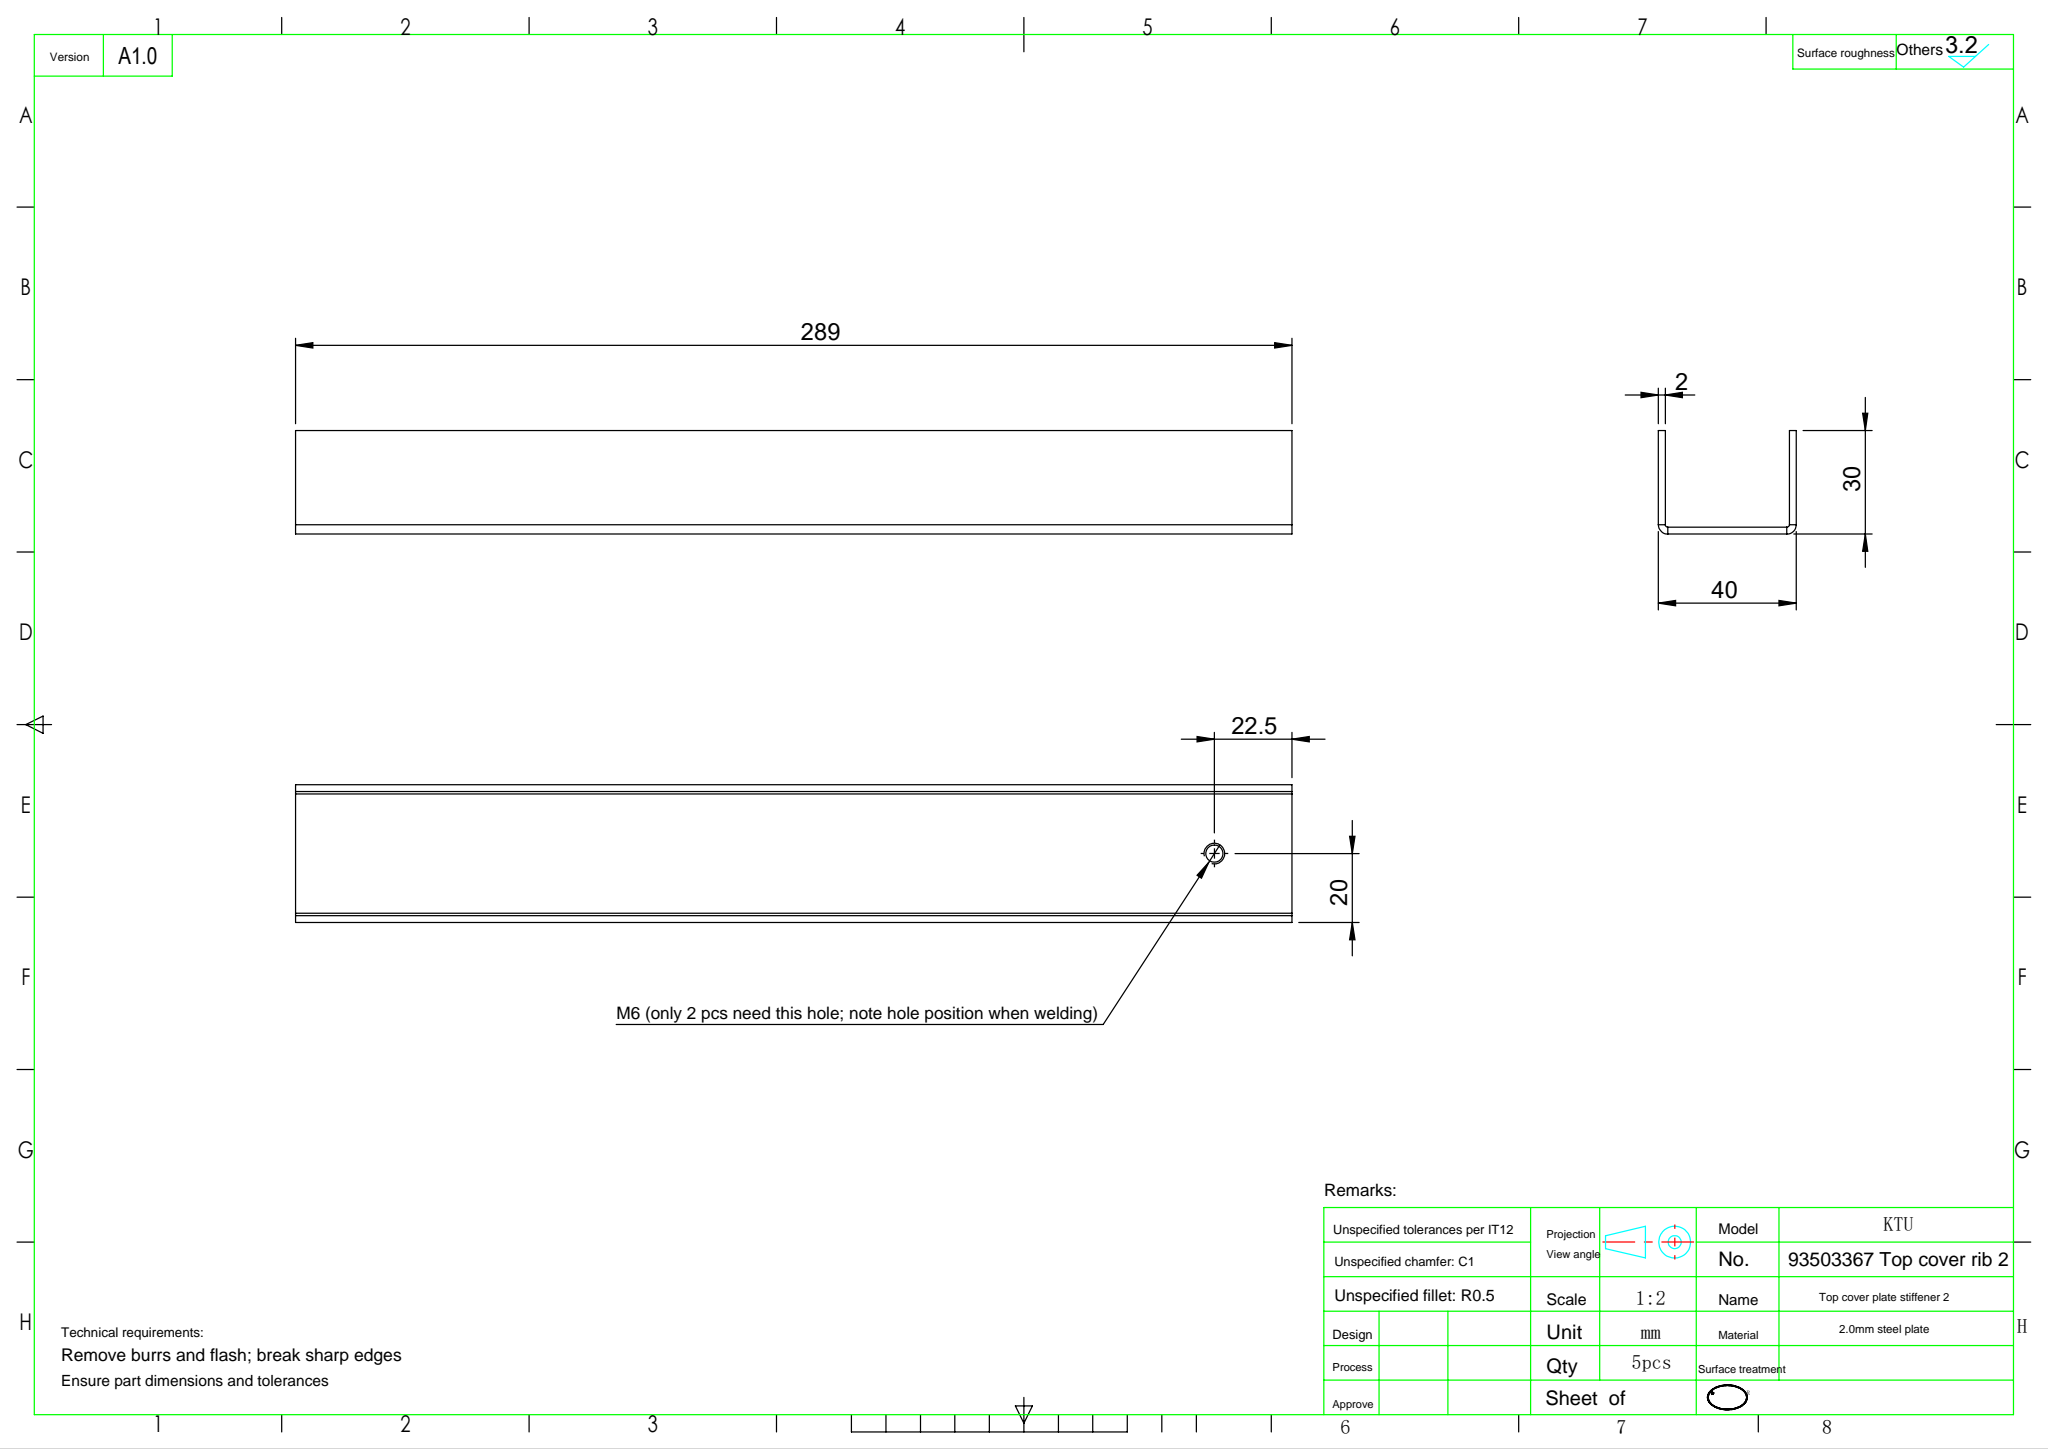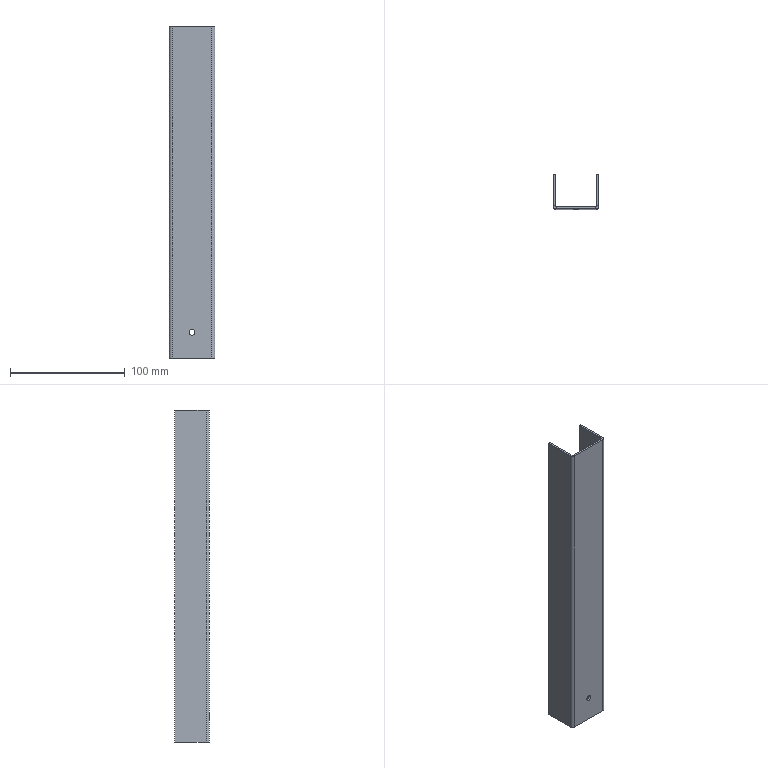Part | SolidWorks | features Cut 1, FlatPattern 1, SMBaseFlange 1, SheetMetal 1 | 1 solid | 24 faces | box 40 x 30 x 289 mm | volume 54587 mm3 | plane 18 | cylinder 6 | commonest cylinder face diameters 1.473 x2 5 x2 5.473 x2
STEP:
#1=CARTESIAN_POINT('',(2.5,-15.,-122.));
#2=VERTEX_POINT('',#1);
#3=CARTESIAN_POINT('',(-2.5,-15.,-122.));
#4=VERTEX_POINT('',#3);
#5=CARTESIAN_POINT('',(0.,-15.,-122.));
#6=DIRECTION('',(0.,1.,0.));
#7=DIRECTION('',(-1.,0.,0.));
#8=AXIS2_PLACEMENT_3D('',#5,#6,#7);
#9=CIRCLE('',#8,2.5);
#10=EDGE_CURVE('',#2,#4,#9,.T.);
#11=ORIENTED_EDGE('',*,*,#10,.F.);
#12=CARTESIAN_POINT('',(2.5,-13.,-122.));
#13=VERTEX_POINT('',#12);
#14=CARTESIAN_POINT('',(2.5,-23.,-122.));
#15=DIRECTION('',(0.,1.,0.));
#16=VECTOR('',#15,1000.);
#17=LINE('',#14,#16);
#18=EDGE_CURVE('',#2,#13,#17,.T.);
#19=ORIENTED_EDGE('',*,*,#18,.T.);
#20=CARTESIAN_POINT('',(-2.5,-13.,-122.));
#21=VERTEX_POINT('',#20);
#22=CARTESIAN_POINT('',(0.,-13.,-122.));
#23=DIRECTION('',(0.,1.,0.));
#24=DIRECTION('',(-1.,0.,0.));
#25=AXIS2_PLACEMENT_3D('',#22,#23,#24);
#26=CIRCLE('',#25,2.5);
#27=EDGE_CURVE('',#13,#21,#26,.T.);
#28=ORIENTED_EDGE('',*,*,#27,.T.);
#29=CARTESIAN_POINT('',(-2.5,-23.,-122.));
#30=DIRECTION('',(0.,1.,0.));
#31=VECTOR('',#30,1000.);
#32=LINE('',#29,#31);
#33=EDGE_CURVE('',#4,#21,#32,.T.);
#34=ORIENTED_EDGE('',*,*,#33,.F.);
#35=EDGE_LOOP('',(#11,#19,#28,#34));
#36=FACE_OUTER_BOUND('',#35,.T.);
#37=CARTESIAN_POINT('',(0.,-23.,-122.));
#38=DIRECTION('',(0.,1.,0.));
#39=DIRECTION('',(-1.,0.,0.));
#40=AXIS2_PLACEMENT_3D('',#37,#38,#39);
#41=CYLINDRICAL_SURFACE('',#40,2.5);
#42=ADVANCED_FACE('',(#36),#41,.F.);
#43=CARTESIAN_POINT('',(-20.,-12.263,144.5));
#44=VERTEX_POINT('',#43);
#45=CARTESIAN_POINT('',(-18.,-12.263,144.5));
#46=VERTEX_POINT('',#45);
#47=CARTESIAN_POINT('',(-20.,-12.263,144.5));
#48=DIRECTION('',(1.,0.,0.));
#49=VECTOR('',#48,1000.);
#50=LINE('',#47,#49);
#51=EDGE_CURVE('',#44,#46,#50,.T.);
#52=ORIENTED_EDGE('',*,*,#51,.F.);
#53=CARTESIAN_POINT('',(-17.263,-15.,144.5));
#54=VERTEX_POINT('',#53);
#55=CARTESIAN_POINT('',(-17.263,-12.263,144.5));
#56=DIRECTION('',(0.,0.,1.));
#57=DIRECTION('',(-1.,0.,0.));
#58=AXIS2_PLACEMENT_3D('',#55,#56,#57);
#59=CIRCLE('',#58,2.737);
#60=EDGE_CURVE('',#44,#54,#59,.T.);
#61=ORIENTED_EDGE('',*,*,#60,.T.);
#62=CARTESIAN_POINT('',(-17.263,-13.,144.5));
#63=VERTEX_POINT('',#62);
#64=CARTESIAN_POINT('',(-17.263,-13.,144.5));
#65=DIRECTION('',(0.,-1.,0.));
#66=VECTOR('',#65,1000.);
#67=LINE('',#64,#66);
#68=EDGE_CURVE('',#63,#54,#67,.T.);
#69=ORIENTED_EDGE('',*,*,#68,.F.);
#70=CARTESIAN_POINT('',(-17.263,-12.263,144.5));
#71=DIRECTION('',(0.,0.,1.));
#72=DIRECTION('',(1.,0.,0.));
#73=AXIS2_PLACEMENT_3D('',#70,#71,#72);
#74=CIRCLE('',#73,0.7366);
#75=EDGE_CURVE('',#46,#63,#74,.T.);
#76=ORIENTED_EDGE('',*,*,#75,.F.);
#77=EDGE_LOOP('',(#52,#61,#69,#76));
#78=FACE_OUTER_BOUND('',#77,.T.);
#79=CARTESIAN_POINT('',(-20.,-12.263,144.5));
#80=DIRECTION('',(0.,0.,1.));
#81=DIRECTION('',(1.,0.,0.));
#82=AXIS2_PLACEMENT_3D('',#79,#80,#81);
#83=PLANE('',#82);
#84=ADVANCED_FACE('',(#78),#83,.T.);
#85=CARTESIAN_POINT('',(-20.,15.,144.5));
#86=VERTEX_POINT('',#85);
#87=CARTESIAN_POINT('',(-20.,-15.,144.5));
#88=DIRECTION('',(0.,-1.,0.));
#89=VECTOR('',#88,1000.);
#90=LINE('',#87,#89);
#91=EDGE_CURVE('',#86,#44,#90,.T.);
#92=ORIENTED_EDGE('',*,*,#91,.T.);
#93=ORIENTED_EDGE('',*,*,#51,.T.);
#94=CARTESIAN_POINT('',(-18.,15.,144.5));
#95=VERTEX_POINT('',#94);
#96=CARTESIAN_POINT('',(-18.,-15.,144.5));
#97=DIRECTION('',(0.,-1.,0.));
#98=VECTOR('',#97,1000.);
#99=LINE('',#96,#98);
#100=EDGE_CURVE('',#95,#46,#99,.T.);
#101=ORIENTED_EDGE('',*,*,#100,.F.);
#102=CARTESIAN_POINT('',(-20.,15.,144.5));
#103=DIRECTION('',(1.,0.,0.));
#104=VECTOR('',#103,1000.);
#105=LINE('',#102,#104);
#106=EDGE_CURVE('',#86,#95,#105,.T.);
#107=ORIENTED_EDGE('',*,*,#106,.F.);
#108=EDGE_LOOP('',(#92,#93,#101,#107));
#109=FACE_OUTER_BOUND('',#108,.T.);
#110=CARTESIAN_POINT('',(-17.263,-13.,144.5));
#111=DIRECTION('',(0.,0.,1.));
#112=DIRECTION('',(1.,0.,0.));
#113=AXIS2_PLACEMENT_3D('',#110,#111,#112);
#114=PLANE('',#113);
#115=ADVANCED_FACE('',(#109),#114,.T.);
#116=CARTESIAN_POINT('',(-17.263,-15.,-144.5));
#117=VERTEX_POINT('',#116);
#118=CARTESIAN_POINT('',(-17.263,-13.,-144.5));
#119=VERTEX_POINT('',#118);
#120=CARTESIAN_POINT('',(-17.263,-15.,-144.5));
#121=DIRECTION('',(0.,1.,0.));
#122=VECTOR('',#121,1000.);
#123=LINE('',#120,#122);
#124=EDGE_CURVE('',#117,#119,#123,.T.);
#125=ORIENTED_EDGE('',*,*,#124,.F.);
#126=CARTESIAN_POINT('',(-20.,-12.263,-144.5));
#127=VERTEX_POINT('',#126);
#128=CARTESIAN_POINT('',(-17.263,-12.263,-144.5));
#129=DIRECTION('',(0.,0.,1.));
#130=DIRECTION('',(-1.,0.,0.));
#131=AXIS2_PLACEMENT_3D('',#128,#129,#130);
#132=CIRCLE('',#131,2.737);
#133=EDGE_CURVE('',#127,#117,#132,.T.);
#134=ORIENTED_EDGE('',*,*,#133,.F.);
#135=CARTESIAN_POINT('',(-18.,-12.263,-144.5));
#136=VERTEX_POINT('',#135);
#137=CARTESIAN_POINT('',(-18.,-12.263,-144.5));
#138=DIRECTION('',(-1.,0.,0.));
#139=VECTOR('',#138,1000.);
#140=LINE('',#137,#139);
#141=EDGE_CURVE('',#136,#127,#140,.T.);
#142=ORIENTED_EDGE('',*,*,#141,.F.);
#143=CARTESIAN_POINT('',(-17.263,-12.263,-144.5));
#144=DIRECTION('',(0.,0.,1.));
#145=DIRECTION('',(1.,0.,0.));
#146=AXIS2_PLACEMENT_3D('',#143,#144,#145);
#147=CIRCLE('',#146,0.7366);
#148=EDGE_CURVE('',#136,#119,#147,.T.);
#149=ORIENTED_EDGE('',*,*,#148,.T.);
#150=EDGE_LOOP('',(#125,#134,#142,#149));
#151=FACE_OUTER_BOUND('',#150,.T.);
#152=CARTESIAN_POINT('',(-17.263,-15.,-144.5));
#153=DIRECTION('',(0.,0.,-1.));
#154=DIRECTION('',(-1.,0.,0.));
#155=AXIS2_PLACEMENT_3D('',#152,#153,#154);
#156=PLANE('',#155);
#157=ADVANCED_FACE('',(#151),#156,.T.);
#158=CARTESIAN_POINT('',(17.263,-15.,-144.5));
#159=VERTEX_POINT('',#158);
#160=CARTESIAN_POINT('',(20.,-15.,-144.5));
#161=DIRECTION('',(1.,0.,0.));
#162=VECTOR('',#161,1000.);
#163=LINE('',#160,#162);
#164=EDGE_CURVE('',#117,#159,#163,.T.);
#165=ORIENTED_EDGE('',*,*,#164,.F.);
#166=ORIENTED_EDGE('',*,*,#124,.T.);
#167=CARTESIAN_POINT('',(17.263,-13.,-144.5));
#168=VERTEX_POINT('',#167);
#169=CARTESIAN_POINT('',(20.,-13.,-144.5));
#170=DIRECTION('',(1.,0.,0.));
#171=VECTOR('',#170,1000.);
#172=LINE('',#169,#171);
#173=EDGE_CURVE('',#119,#168,#172,.T.);
#174=ORIENTED_EDGE('',*,*,#173,.T.);
#175=CARTESIAN_POINT('',(17.263,-13.,-144.5));
#176=DIRECTION('',(0.,-1.,0.));
#177=VECTOR('',#176,1000.);
#178=LINE('',#175,#177);
#179=EDGE_CURVE('',#168,#159,#178,.T.);
#180=ORIENTED_EDGE('',*,*,#179,.T.);
#181=EDGE_LOOP('',(#165,#166,#174,#180));
#182=FACE_OUTER_BOUND('',#181,.T.);
#183=CARTESIAN_POINT('',(-18.,-12.263,-144.5));
#184=DIRECTION('',(0.,0.,-1.));
#185=DIRECTION('',(-1.,0.,0.));
#186=AXIS2_PLACEMENT_3D('',#183,#184,#185);
#187=PLANE('',#186);
#188=ADVANCED_FACE('',(#182),#187,.T.);
#189=CARTESIAN_POINT('',(17.263,-15.,144.5));
#190=VERTEX_POINT('',#189);
#191=CARTESIAN_POINT('',(17.263,-13.,144.5));
#192=VERTEX_POINT('',#191);
#193=CARTESIAN_POINT('',(17.263,-15.,144.5));
#194=DIRECTION('',(0.,1.,0.));
#195=VECTOR('',#194,1000.);
#196=LINE('',#193,#195);
#197=EDGE_CURVE('',#190,#192,#196,.T.);
#198=ORIENTED_EDGE('',*,*,#197,.F.);
#199=CARTESIAN_POINT('',(20.,-12.263,144.5));
#200=VERTEX_POINT('',#199);
#201=CARTESIAN_POINT('',(17.263,-12.263,144.5));
#202=DIRECTION('',(0.,0.,1.));
#203=DIRECTION('',(-1.,0.,0.));
#204=AXIS2_PLACEMENT_3D('',#201,#202,#203);
#205=CIRCLE('',#204,2.737);
#206=EDGE_CURVE('',#190,#200,#205,.T.);
#207=ORIENTED_EDGE('',*,*,#206,.T.);
#208=CARTESIAN_POINT('',(18.,-12.263,144.5));
#209=VERTEX_POINT('',#208);
#210=CARTESIAN_POINT('',(18.,-12.263,144.5));
#211=DIRECTION('',(1.,0.,0.));
#212=VECTOR('',#211,1000.);
#213=LINE('',#210,#212);
#214=EDGE_CURVE('',#209,#200,#213,.T.);
#215=ORIENTED_EDGE('',*,*,#214,.F.);
#216=CARTESIAN_POINT('',(17.263,-12.263,144.5));
#217=DIRECTION('',(0.,0.,1.));
#218=DIRECTION('',(1.,0.,0.));
#219=AXIS2_PLACEMENT_3D('',#216,#217,#218);
#220=CIRCLE('',#219,0.7366);
#221=EDGE_CURVE('',#192,#209,#220,.T.);
#222=ORIENTED_EDGE('',*,*,#221,.F.);
#223=EDGE_LOOP('',(#198,#207,#215,#222));
#224=FACE_OUTER_BOUND('',#223,.T.);
#225=CARTESIAN_POINT('',(17.263,-15.,144.5));
#226=DIRECTION('',(0.,0.,1.));
#227=DIRECTION('',(1.,0.,0.));
#228=AXIS2_PLACEMENT_3D('',#225,#226,#227);
#229=PLANE('',#228);
#230=ADVANCED_FACE('',(#224),#229,.T.);
#231=CARTESIAN_POINT('',(20.,-15.,144.5));
#232=DIRECTION('',(1.,0.,0.));
#233=VECTOR('',#232,1000.);
#234=LINE('',#231,#233);
#235=EDGE_CURVE('',#54,#190,#234,.T.);
#236=ORIENTED_EDGE('',*,*,#235,.T.);
#237=ORIENTED_EDGE('',*,*,#197,.T.);
#238=CARTESIAN_POINT('',(20.,-13.,144.5));
#239=DIRECTION('',(1.,0.,0.));
#240=VECTOR('',#239,1000.);
#241=LINE('',#238,#240);
#242=EDGE_CURVE('',#63,#192,#241,.T.);
#243=ORIENTED_EDGE('',*,*,#242,.F.);
#244=ORIENTED_EDGE('',*,*,#68,.T.);
#245=EDGE_LOOP('',(#236,#237,#243,#244));
#246=FACE_OUTER_BOUND('',#245,.T.);
#247=CARTESIAN_POINT('',(18.,-12.263,144.5));
#248=DIRECTION('',(0.,0.,1.));
#249=DIRECTION('',(1.,0.,0.));
#250=AXIS2_PLACEMENT_3D('',#247,#248,#249);
#251=PLANE('',#250);
#252=ADVANCED_FACE('',(#246),#251,.T.);
#253=CARTESIAN_POINT('',(20.,-12.263,-144.5));
#254=VERTEX_POINT('',#253);
#255=CARTESIAN_POINT('',(18.,-12.263,-144.5));
#256=VERTEX_POINT('',#255);
#257=CARTESIAN_POINT('',(20.,-12.263,-144.5));
#258=DIRECTION('',(-1.,0.,0.));
#259=VECTOR('',#258,1000.);
#260=LINE('',#257,#259);
#261=EDGE_CURVE('',#254,#256,#260,.T.);
#262=ORIENTED_EDGE('',*,*,#261,.F.);
#263=CARTESIAN_POINT('',(17.263,-12.263,-144.5));
#264=DIRECTION('',(0.,0.,1.));
#265=DIRECTION('',(-1.,0.,0.));
#266=AXIS2_PLACEMENT_3D('',#263,#264,#265);
#267=CIRCLE('',#266,2.737);
#268=EDGE_CURVE('',#159,#254,#267,.T.);
#269=ORIENTED_EDGE('',*,*,#268,.F.);
#270=ORIENTED_EDGE('',*,*,#179,.F.);
#271=CARTESIAN_POINT('',(17.263,-12.263,-144.5));
#272=DIRECTION('',(0.,0.,1.));
#273=DIRECTION('',(1.,0.,0.));
#274=AXIS2_PLACEMENT_3D('',#271,#272,#273);
#275=CIRCLE('',#274,0.7366);
#276=EDGE_CURVE('',#168,#256,#275,.T.);
#277=ORIENTED_EDGE('',*,*,#276,.T.);
#278=EDGE_LOOP('',(#262,#269,#270,#277));
#279=FACE_OUTER_BOUND('',#278,.T.);
#280=CARTESIAN_POINT('',(20.,-12.263,-144.5));
#281=DIRECTION('',(0.,0.,-1.));
#282=DIRECTION('',(-1.,0.,0.));
#283=AXIS2_PLACEMENT_3D('',#280,#281,#282);
#284=PLANE('',#283);
#285=ADVANCED_FACE('',(#279),#284,.T.);
#286=CARTESIAN_POINT('',(20.,15.,-144.5));
#287=VERTEX_POINT('',#286);
#288=CARTESIAN_POINT('',(20.,-15.,-144.5));
#289=DIRECTION('',(0.,1.,0.));
#290=VECTOR('',#289,1000.);
#291=LINE('',#288,#290);
#292=EDGE_CURVE('',#254,#287,#291,.T.);
#293=ORIENTED_EDGE('',*,*,#292,.F.);
#294=ORIENTED_EDGE('',*,*,#261,.T.);
#295=CARTESIAN_POINT('',(18.,15.,-144.5));
#296=VERTEX_POINT('',#295);
#297=CARTESIAN_POINT('',(18.,-15.,-144.5));
#298=DIRECTION('',(0.,1.,0.));
#299=VECTOR('',#298,1000.);
#300=LINE('',#297,#299);
#301=EDGE_CURVE('',#256,#296,#300,.T.);
#302=ORIENTED_EDGE('',*,*,#301,.T.);
#303=CARTESIAN_POINT('',(18.,15.,-144.5));
#304=DIRECTION('',(1.,0.,0.));
#305=VECTOR('',#304,1000.);
#306=LINE('',#303,#305);
#307=EDGE_CURVE('',#296,#287,#306,.T.);
#308=ORIENTED_EDGE('',*,*,#307,.T.);
#309=EDGE_LOOP('',(#293,#294,#302,#308));
#310=FACE_OUTER_BOUND('',#309,.T.);
#311=CARTESIAN_POINT('',(17.263,-13.,-144.5));
#312=DIRECTION('',(0.,0.,-1.));
#313=DIRECTION('',(-1.,0.,0.));
#314=AXIS2_PLACEMENT_3D('',#311,#312,#313);
#315=PLANE('',#314);
#316=ADVANCED_FACE('',(#310),#315,.T.);
#317=ORIENTED_EDGE('',*,*,#292,.T.);
#318=CARTESIAN_POINT('',(20.,15.,144.5));
#319=VERTEX_POINT('',#318);
#320=CARTESIAN_POINT('',(20.,15.,144.5));
#321=DIRECTION('',(0.,0.,-1.));
#322=VECTOR('',#321,1000.);
#323=LINE('',#320,#322);
#324=EDGE_CURVE('',#319,#287,#323,.T.);
#325=ORIENTED_EDGE('',*,*,#324,.F.);
#326=CARTESIAN_POINT('',(20.,-15.,144.5));
#327=DIRECTION('',(0.,1.,0.));
#328=VECTOR('',#327,1000.);
#329=LINE('',#326,#328);
#330=EDGE_CURVE('',#200,#319,#329,.T.);
#331=ORIENTED_EDGE('',*,*,#330,.F.);
#332=CARTESIAN_POINT('',(20.,-12.263,144.5));
#333=DIRECTION('',(0.,0.,-1.));
#334=VECTOR('',#333,1000.);
#335=LINE('',#332,#334);
#336=EDGE_CURVE('',#200,#254,#335,.T.);
#337=ORIENTED_EDGE('',*,*,#336,.T.);
#338=EDGE_LOOP('',(#317,#325,#331,#337));
#339=FACE_OUTER_BOUND('',#338,.T.);
#340=CARTESIAN_POINT('',(20.,-15.,144.5));
#341=DIRECTION('',(-1.,0.,0.));
#342=DIRECTION('',(0.,0.,1.));
#343=AXIS2_PLACEMENT_3D('',#340,#341,#342);
#344=PLANE('',#343);
#345=ADVANCED_FACE('',(#339),#344,.F.);
#346=ORIENTED_EDGE('',*,*,#307,.F.);
#347=CARTESIAN_POINT('',(18.,15.,144.5));
#348=VERTEX_POINT('',#347);
#349=CARTESIAN_POINT('',(18.,15.,144.5));
#350=DIRECTION('',(0.,0.,-1.));
#351=VECTOR('',#350,1000.);
#352=LINE('',#349,#351);
#353=EDGE_CURVE('',#348,#296,#352,.T.);
#354=ORIENTED_EDGE('',*,*,#353,.F.);
#355=CARTESIAN_POINT('',(18.,15.,144.5));
#356=DIRECTION('',(1.,0.,0.));
#357=VECTOR('',#356,1000.);
#358=LINE('',#355,#357);
#359=EDGE_CURVE('',#348,#319,#358,.T.);
#360=ORIENTED_EDGE('',*,*,#359,.T.);
#361=ORIENTED_EDGE('',*,*,#324,.T.);
#362=EDGE_LOOP('',(#346,#354,#360,#361));
#363=FACE_OUTER_BOUND('',#362,.T.);
#364=CARTESIAN_POINT('',(18.,15.,144.5));
#365=DIRECTION('',(0.,1.,0.));
#366=DIRECTION('',(-1.,0.,0.));
#367=AXIS2_PLACEMENT_3D('',#364,#365,#366);
#368=PLANE('',#367);
#369=ADVANCED_FACE('',(#363),#368,.T.);
#370=ORIENTED_EDGE('',*,*,#301,.F.);
#371=CARTESIAN_POINT('',(18.,-12.263,144.5));
#372=DIRECTION('',(0.,0.,-1.));
#373=VECTOR('',#372,1000.);
#374=LINE('',#371,#373);
#375=EDGE_CURVE('',#209,#256,#374,.T.);
#376=ORIENTED_EDGE('',*,*,#375,.F.);
#377=CARTESIAN_POINT('',(18.,-15.,144.5));
#378=DIRECTION('',(0.,1.,0.));
#379=VECTOR('',#378,1000.);
#380=LINE('',#377,#379);
#381=EDGE_CURVE('',#209,#348,#380,.T.);
#382=ORIENTED_EDGE('',*,*,#381,.T.);
#383=ORIENTED_EDGE('',*,*,#353,.T.);
#384=EDGE_LOOP('',(#370,#376,#382,#383));
#385=FACE_OUTER_BOUND('',#384,.T.);
#386=CARTESIAN_POINT('',(18.,-15.,144.5));
#387=DIRECTION('',(-1.,0.,0.));
#388=DIRECTION('',(0.,0.,1.));
#389=AXIS2_PLACEMENT_3D('',#386,#387,#388);
#390=PLANE('',#389);
#391=ADVANCED_FACE('',(#385),#390,.T.);
#392=ORIENTED_EDGE('',*,*,#276,.F.);
#393=CARTESIAN_POINT('',(17.263,-13.,144.5));
#394=DIRECTION('',(0.,0.,-1.));
#395=VECTOR('',#394,1000.);
#396=LINE('',#393,#395);
#397=EDGE_CURVE('',#192,#168,#396,.T.);
#398=ORIENTED_EDGE('',*,*,#397,.F.);
#399=ORIENTED_EDGE('',*,*,#221,.T.);
#400=ORIENTED_EDGE('',*,*,#375,.T.);
#401=EDGE_LOOP('',(#392,#398,#399,#400));
#402=FACE_OUTER_BOUND('',#401,.T.);
#403=CARTESIAN_POINT('',(17.263,-12.263,144.5));
#404=DIRECTION('',(0.,0.,-1.));
#405=DIRECTION('',(-1.,0.,0.));
#406=AXIS2_PLACEMENT_3D('',#403,#404,#405);
#407=CYLINDRICAL_SURFACE('',#406,0.7366);
#408=ADVANCED_FACE('',(#402),#407,.F.);
#409=CARTESIAN_POINT('',(0.,-13.,-122.));
#410=DIRECTION('',(0.,1.,0.));
#411=DIRECTION('',(-1.,0.,0.));
#412=AXIS2_PLACEMENT_3D('',#409,#410,#411);
#413=CIRCLE('',#412,2.5);
#414=EDGE_CURVE('',#21,#13,#413,.T.);
#415=ORIENTED_EDGE('',*,*,#414,.F.);
#416=ORIENTED_EDGE('',*,*,#27,.F.);
#417=EDGE_LOOP('',(#415,#416));
#418=FACE_BOUND('',#417,.T.);
#419=ORIENTED_EDGE('',*,*,#173,.F.);
#420=CARTESIAN_POINT('',(-17.263,-13.,144.5));
#421=DIRECTION('',(0.,0.,-1.));
#422=VECTOR('',#421,1000.);
#423=LINE('',#420,#422);
#424=EDGE_CURVE('',#63,#119,#423,.T.);
#425=ORIENTED_EDGE('',*,*,#424,.F.);
#426=ORIENTED_EDGE('',*,*,#242,.T.);
#427=ORIENTED_EDGE('',*,*,#397,.T.);
#428=EDGE_LOOP('',(#419,#425,#426,#427));
#429=FACE_OUTER_BOUND('',#428,.T.);
#430=CARTESIAN_POINT('',(20.,-13.,144.5));
#431=DIRECTION('',(0.,1.,0.));
#432=DIRECTION('',(-1.,0.,0.));
#433=AXIS2_PLACEMENT_3D('',#430,#431,#432);
#434=PLANE('',#433);
#435=ADVANCED_FACE('',(#418,#429),#434,.T.);
#436=ORIENTED_EDGE('',*,*,#148,.F.);
#437=CARTESIAN_POINT('',(-18.,-12.263,144.5));
#438=DIRECTION('',(0.,0.,-1.));
#439=VECTOR('',#438,1000.);
#440=LINE('',#437,#439);
#441=EDGE_CURVE('',#46,#136,#440,.T.);
#442=ORIENTED_EDGE('',*,*,#441,.F.);
#443=ORIENTED_EDGE('',*,*,#75,.T.);
#444=ORIENTED_EDGE('',*,*,#424,.T.);
#445=EDGE_LOOP('',(#436,#442,#443,#444));
#446=FACE_OUTER_BOUND('',#445,.T.);
#447=CARTESIAN_POINT('',(-17.263,-12.263,144.5));
#448=DIRECTION('',(0.,0.,-1.));
#449=DIRECTION('',(-1.,0.,0.));
#450=AXIS2_PLACEMENT_3D('',#447,#448,#449);
#451=CYLINDRICAL_SURFACE('',#450,0.7366);
#452=ADVANCED_FACE('',(#446),#451,.F.);
#453=CARTESIAN_POINT('',(-18.,15.,-144.5));
#454=VERTEX_POINT('',#453);
#455=CARTESIAN_POINT('',(-18.,-15.,-144.5));
#456=DIRECTION('',(0.,-1.,0.));
#457=VECTOR('',#456,1000.);
#458=LINE('',#455,#457);
#459=EDGE_CURVE('',#454,#136,#458,.T.);
#460=ORIENTED_EDGE('',*,*,#459,.F.);
#461=CARTESIAN_POINT('',(-18.,15.,144.5));
#462=DIRECTION('',(0.,0.,-1.));
#463=VECTOR('',#462,1000.);
#464=LINE('',#461,#463);
#465=EDGE_CURVE('',#95,#454,#464,.T.);
#466=ORIENTED_EDGE('',*,*,#465,.F.);
#467=ORIENTED_EDGE('',*,*,#100,.T.);
#468=ORIENTED_EDGE('',*,*,#441,.T.);
#469=EDGE_LOOP('',(#460,#466,#467,#468));
#470=FACE_OUTER_BOUND('',#469,.T.);
#471=CARTESIAN_POINT('',(-18.,-15.,144.5));
#472=DIRECTION('',(1.,0.,0.));
#473=DIRECTION('',(0.,0.,-1.));
#474=AXIS2_PLACEMENT_3D('',#471,#472,#473);
#475=PLANE('',#474);
#476=ADVANCED_FACE('',(#470),#475,.T.);
#477=CARTESIAN_POINT('',(-20.,15.,-144.5));
#478=VERTEX_POINT('',#477);
#479=CARTESIAN_POINT('',(-20.,15.,-144.5));
#480=DIRECTION('',(1.,0.,0.));
#481=VECTOR('',#480,1000.);
#482=LINE('',#479,#481);
#483=EDGE_CURVE('',#478,#454,#482,.T.);
#484=ORIENTED_EDGE('',*,*,#483,.F.);
#485=CARTESIAN_POINT('',(-20.,15.,144.5));
#486=DIRECTION('',(0.,0.,-1.));
#487=VECTOR('',#486,1000.);
#488=LINE('',#485,#487);
#489=EDGE_CURVE('',#86,#478,#488,.T.);
#490=ORIENTED_EDGE('',*,*,#489,.F.);
#491=ORIENTED_EDGE('',*,*,#106,.T.);
#492=ORIENTED_EDGE('',*,*,#465,.T.);
#493=EDGE_LOOP('',(#484,#490,#491,#492));
#494=FACE_OUTER_BOUND('',#493,.T.);
#495=CARTESIAN_POINT('',(-20.,15.,144.5));
#496=DIRECTION('',(0.,1.,0.));
#497=DIRECTION('',(-1.,0.,0.));
#498=AXIS2_PLACEMENT_3D('',#495,#496,#497);
#499=PLANE('',#498);
#500=ADVANCED_FACE('',(#494),#499,.T.);
#501=CARTESIAN_POINT('',(-20.,-15.,-144.5));
#502=DIRECTION('',(0.,-1.,0.));
#503=VECTOR('',#502,1000.);
#504=LINE('',#501,#503);
#505=EDGE_CURVE('',#478,#127,#504,.T.);
#506=ORIENTED_EDGE('',*,*,#505,.T.);
#507=CARTESIAN_POINT('',(-20.,-12.263,144.5));
#508=DIRECTION('',(0.,0.,-1.));
#509=VECTOR('',#508,1000.);
#510=LINE('',#507,#509);
#511=EDGE_CURVE('',#44,#127,#510,.T.);
#512=ORIENTED_EDGE('',*,*,#511,.F.);
#513=ORIENTED_EDGE('',*,*,#91,.F.);
#514=ORIENTED_EDGE('',*,*,#489,.T.);
#515=EDGE_LOOP('',(#506,#512,#513,#514));
#516=FACE_OUTER_BOUND('',#515,.T.);
#517=CARTESIAN_POINT('',(-20.,-15.,144.5));
#518=DIRECTION('',(1.,0.,0.));
#519=DIRECTION('',(0.,0.,-1.));
#520=AXIS2_PLACEMENT_3D('',#517,#518,#519);
#521=PLANE('',#520);
#522=ADVANCED_FACE('',(#516),#521,.F.);
#523=ORIENTED_EDGE('',*,*,#133,.T.);
#524=CARTESIAN_POINT('',(-17.263,-15.,144.5));
#525=DIRECTION('',(0.,0.,-1.));
#526=VECTOR('',#525,1000.);
#527=LINE('',#524,#526);
#528=EDGE_CURVE('',#54,#117,#527,.T.);
#529=ORIENTED_EDGE('',*,*,#528,.F.);
#530=ORIENTED_EDGE('',*,*,#60,.F.);
#531=ORIENTED_EDGE('',*,*,#511,.T.);
#532=EDGE_LOOP('',(#523,#529,#530,#531));
#533=FACE_OUTER_BOUND('',#532,.T.);
#534=CARTESIAN_POINT('',(-17.263,-12.263,144.5));
#535=DIRECTION('',(0.,0.,-1.));
#536=DIRECTION('',(-1.,0.,0.));
#537=AXIS2_PLACEMENT_3D('',#534,#535,#536);
#538=CYLINDRICAL_SURFACE('',#537,2.737);
#539=ADVANCED_FACE('',(#533),#538,.T.);
#540=CARTESIAN_POINT('',(0.,-15.,-122.));
#541=DIRECTION('',(0.,1.,0.));
#542=DIRECTION('',(-1.,0.,0.));
#543=AXIS2_PLACEMENT_3D('',#540,#541,#542);
#544=CIRCLE('',#543,2.5);
#545=EDGE_CURVE('',#4,#2,#544,.T.);
#546=ORIENTED_EDGE('',*,*,#545,.T.);
#547=ORIENTED_EDGE('',*,*,#10,.T.);
#548=EDGE_LOOP('',(#546,#547));
#549=FACE_BOUND('',#548,.T.);
#550=ORIENTED_EDGE('',*,*,#164,.T.);
#551=CARTESIAN_POINT('',(17.263,-15.,144.5));
#552=DIRECTION('',(0.,0.,-1.));
#553=VECTOR('',#552,1000.);
#554=LINE('',#551,#553);
#555=EDGE_CURVE('',#190,#159,#554,.T.);
#556=ORIENTED_EDGE('',*,*,#555,.F.);
#557=ORIENTED_EDGE('',*,*,#235,.F.);
#558=ORIENTED_EDGE('',*,*,#528,.T.);
#559=EDGE_LOOP('',(#550,#556,#557,#558));
#560=FACE_OUTER_BOUND('',#559,.T.);
#561=CARTESIAN_POINT('',(20.,-15.,144.5));
#562=DIRECTION('',(0.,1.,0.));
#563=DIRECTION('',(-1.,0.,0.));
#564=AXIS2_PLACEMENT_3D('',#561,#562,#563);
#565=PLANE('',#564);
#566=ADVANCED_FACE('',(#549,#560),#565,.F.);
#567=ORIENTED_EDGE('',*,*,#268,.T.);
#568=ORIENTED_EDGE('',*,*,#336,.F.);
#569=ORIENTED_EDGE('',*,*,#206,.F.);
#570=ORIENTED_EDGE('',*,*,#555,.T.);
#571=EDGE_LOOP('',(#567,#568,#569,#570));
#572=FACE_OUTER_BOUND('',#571,.T.);
#573=CARTESIAN_POINT('',(17.263,-12.263,144.5));
#574=DIRECTION('',(0.,0.,-1.));
#575=DIRECTION('',(-1.,0.,0.));
#576=AXIS2_PLACEMENT_3D('',#573,#574,#575);
#577=CYLINDRICAL_SURFACE('',#576,2.737);
#578=ADVANCED_FACE('',(#572),#577,.T.);
#579=ORIENTED_EDGE('',*,*,#330,.T.);
#580=ORIENTED_EDGE('',*,*,#359,.F.);
#581=ORIENTED_EDGE('',*,*,#381,.F.);
#582=ORIENTED_EDGE('',*,*,#214,.T.);
#583=EDGE_LOOP('',(#579,#580,#581,#582));
#584=FACE_OUTER_BOUND('',#583,.T.);
#585=CARTESIAN_POINT('',(17.263,-12.263,144.5));
#586=DIRECTION('',(0.,0.,1.));
#587=DIRECTION('',(1.,0.,0.));
#588=AXIS2_PLACEMENT_3D('',#585,#586,#587);
#589=PLANE('',#588);
#590=ADVANCED_FACE('',(#584),#589,.T.);
#591=ORIENTED_EDGE('',*,*,#459,.T.);
#592=ORIENTED_EDGE('',*,*,#141,.T.);
#593=ORIENTED_EDGE('',*,*,#505,.F.);
#594=ORIENTED_EDGE('',*,*,#483,.T.);
#595=EDGE_LOOP('',(#591,#592,#593,#594));
#596=FACE_OUTER_BOUND('',#595,.T.);
#597=CARTESIAN_POINT('',(17.263,-12.263,-144.5));
#598=DIRECTION('',(0.,0.,1.));
#599=DIRECTION('',(1.,0.,0.));
#600=AXIS2_PLACEMENT_3D('',#597,#598,#599);
#601=PLANE('',#600);
#602=ADVANCED_FACE('',(#596),#601,.F.);
#603=ORIENTED_EDGE('',*,*,#18,.F.);
#604=ORIENTED_EDGE('',*,*,#545,.F.);
#605=ORIENTED_EDGE('',*,*,#33,.T.);
#606=ORIENTED_EDGE('',*,*,#414,.T.);
#607=EDGE_LOOP('',(#603,#604,#605,#606));
#608=FACE_OUTER_BOUND('',#607,.T.);
#609=CARTESIAN_POINT('',(0.,-23.,-122.));
#610=DIRECTION('',(0.,1.,0.));
#611=DIRECTION('',(-1.,0.,0.));
#612=AXIS2_PLACEMENT_3D('',#609,#610,#611);
#613=CYLINDRICAL_SURFACE('',#612,2.5);
#614=ADVANCED_FACE('',(#608),#613,.F.);
#615=CLOSED_SHELL('',(#42,#84,#115,#157,#188,#230,#252,#285,#316,#345,#369,#391,#408,#435,#452,#476,#500,#522,#539,#566,#578,#590,#602,#614));
#616=MANIFOLD_SOLID_BREP('',#615);
#617=CARTESIAN_POINT('',(0.,0.,0.));
#618=DIRECTION('',(0.,0.,1.));
#619=DIRECTION('',(1.,0.,0.));
#620=AXIS2_PLACEMENT_3D('',#617,#618,#619);
#621=(LENGTH_UNIT()NAMED_UNIT(*)SI_UNIT(.MILLI.,.METRE.));
#622=UNCERTAINTY_MEASURE_WITH_UNIT(LENGTH_MEASURE(0.00001),#621,'','');
#623=(NAMED_UNIT(*)PLANE_ANGLE_UNIT()SI_UNIT($,.RADIAN.));
#624=(NAMED_UNIT(*)SI_UNIT($,.STERADIAN.)SOLID_ANGLE_UNIT());
#625=(GEOMETRIC_REPRESENTATION_CONTEXT(3)GLOBAL_UNCERTAINTY_ASSIGNED_CONTEXT((#622))GLOBAL_UNIT_ASSIGNED_CONTEXT((#621,#623,#624))REPRESENTATION_CONTEXT('',''));
#626=ADVANCED_BREP_SHAPE_REPRESENTATION('',(#616,#620),#625);